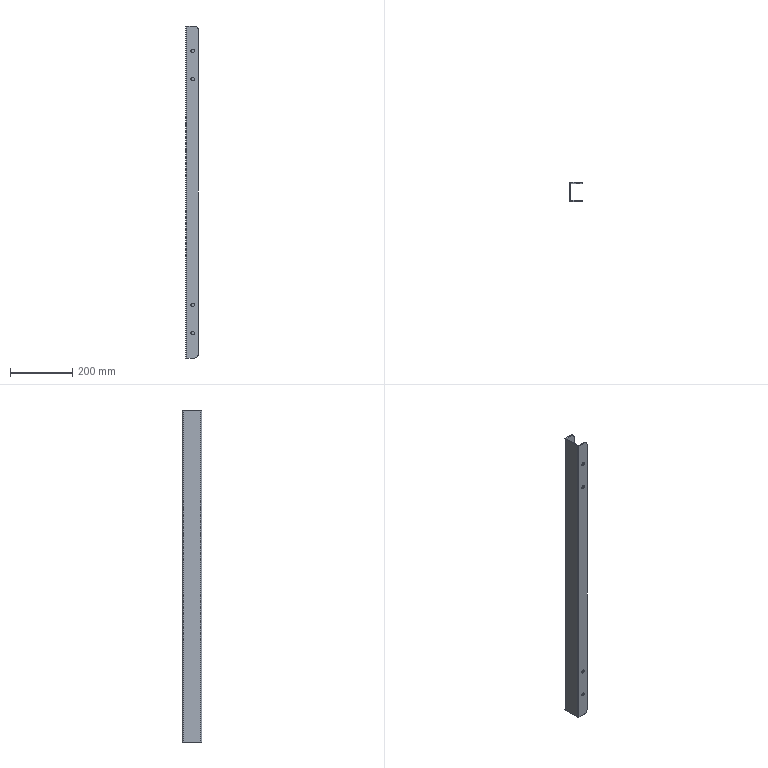Part | 1 solid | 63 faces | box 40 x 62 x 1064 mm | volume 423028 mm3 | cylinder 35 | plane 28 | commonest cylinder face diameters 10 x15 11 x8 12.5 x4 24 x4 0.4 x2 6.4 x2